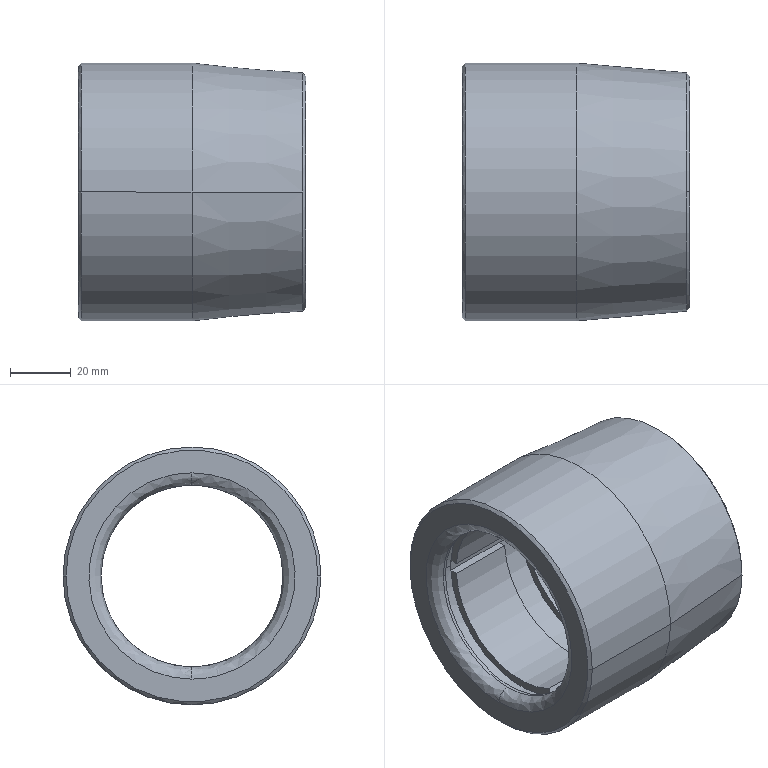Part | SolidWorks | features BaseBody 1 | 1 solid | 64 faces | box 75 x 85 x 85 mm | volume 185357 mm3 | plane 37 | cylinder 19 | cone 6 | spline 2 | commonest cylinder face diameters 60 x10 65 x7 85 x2